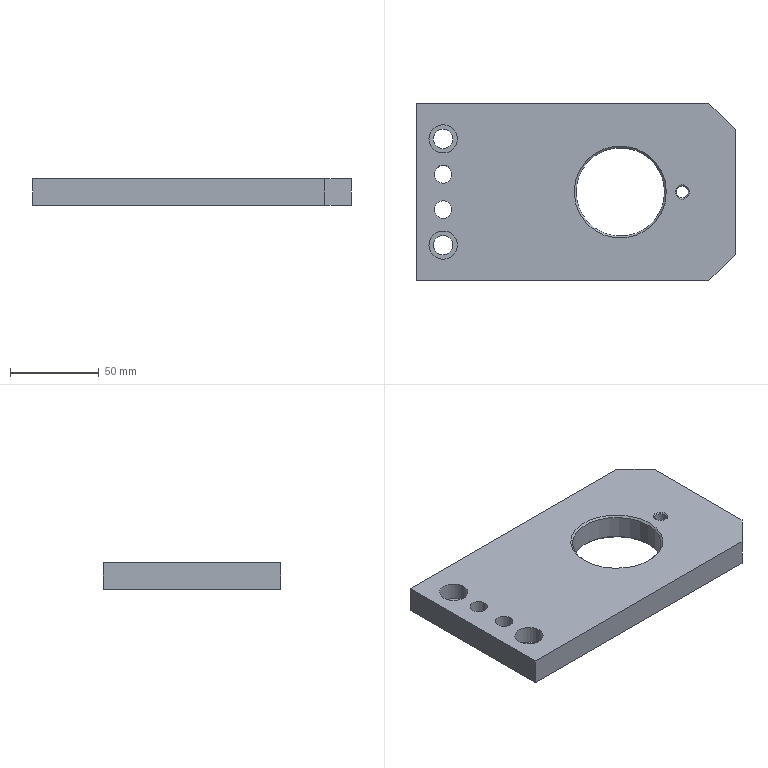Part | NX | features DATUM_CSYS 8, SKETCH 7, HOLE PACKAGE 5, EXTRACT_FACE 4, SIMPLE HOLE 3, CBORE_HOLE 2, CHAMFER 2, EXTRUDE 2, Instance Feature 1, Mirror Feature 1, SYMBOLIC_THREAD 1 | 1 solid | 22 faces | box 180 x 100 x 15 mm | volume 229133 mm3 | plane 10 | cylinder 8 | cone 4 | commonest cylinder face diameters 10 x2 11 x2 16 x2 6.8 x1 50 x1
STEP:
#1=CARTESIAN_POINT('',(0.,100.,0.));
#2=VERTEX_POINT('',#1);
#3=CARTESIAN_POINT('',(0.,0.,0.));
#4=VERTEX_POINT('',#3);
#5=CARTESIAN_POINT('',(0.,100.,0.));
#6=DIRECTION('',(0.,-1.,0.));
#7=VECTOR('',#6,1000.);
#8=LINE('',#5,#7);
#9=EDGE_CURVE('',#2,#4,#8,.T.);
#10=ORIENTED_EDGE('',*,*,#9,.T.);
#11=CARTESIAN_POINT('',(0.,0.,15.));
#12=VERTEX_POINT('',#11);
#13=CARTESIAN_POINT('',(0.,0.,15.));
#14=DIRECTION('',(0.,0.,-1.));
#15=VECTOR('',#14,1000.);
#16=LINE('',#13,#15);
#17=EDGE_CURVE('',#12,#4,#16,.T.);
#18=ORIENTED_EDGE('',*,*,#17,.F.);
#19=CARTESIAN_POINT('',(0.,100.,15.));
#20=VERTEX_POINT('',#19);
#21=CARTESIAN_POINT('',(0.,100.,15.));
#22=DIRECTION('',(0.,-1.,0.));
#23=VECTOR('',#22,1000.);
#24=LINE('',#21,#23);
#25=EDGE_CURVE('',#20,#12,#24,.T.);
#26=ORIENTED_EDGE('',*,*,#25,.F.);
#27=CARTESIAN_POINT('',(0.,100.,15.));
#28=DIRECTION('',(0.,0.,-1.));
#29=VECTOR('',#28,1000.);
#30=LINE('',#27,#29);
#31=EDGE_CURVE('',#20,#2,#30,.T.);
#32=ORIENTED_EDGE('',*,*,#31,.T.);
#33=EDGE_LOOP('',(#10,#18,#26,#32));
#34=FACE_BOUND('',#33,.T.);
#35=CARTESIAN_POINT('',(0.,100.,15.));
#36=DIRECTION('',(1.,0.,0.));
#37=DIRECTION('',(0.,0.,-1.));
#38=AXIS2_PLACEMENT_3D('',#35,#36,#37);
#39=PLANE('',#38);
#40=ADVANCED_FACE('',(#34),#39,.F.);
#41=CARTESIAN_POINT('',(165.,0.,0.));
#42=VERTEX_POINT('',#41);
#43=CARTESIAN_POINT('',(0.,0.,0.));
#44=DIRECTION('',(1.,0.,0.));
#45=VECTOR('',#44,1000.);
#46=LINE('',#43,#45);
#47=EDGE_CURVE('',#4,#42,#46,.T.);
#48=ORIENTED_EDGE('',*,*,#47,.T.);
#49=CARTESIAN_POINT('',(165.,0.,15.));
#50=VERTEX_POINT('',#49);
#51=CARTESIAN_POINT('',(165.,0.,15.));
#52=DIRECTION('',(0.,0.,1.));
#53=VECTOR('',#52,1000.);
#54=LINE('',#51,#53);
#55=EDGE_CURVE('',#42,#50,#54,.T.);
#56=ORIENTED_EDGE('',*,*,#55,.T.);
#57=CARTESIAN_POINT('',(0.,0.,15.));
#58=DIRECTION('',(1.,0.,0.));
#59=VECTOR('',#58,1000.);
#60=LINE('',#57,#59);
#61=EDGE_CURVE('',#12,#50,#60,.T.);
#62=ORIENTED_EDGE('',*,*,#61,.F.);
#63=ORIENTED_EDGE('',*,*,#17,.T.);
#64=EDGE_LOOP('',(#48,#56,#62,#63));
#65=FACE_BOUND('',#64,.T.);
#66=CARTESIAN_POINT('',(0.,0.,15.));
#67=DIRECTION('',(0.,1.,0.));
#68=DIRECTION('',(0.,0.,1.));
#69=AXIS2_PLACEMENT_3D('',#66,#67,#68);
#70=PLANE('',#69);
#71=ADVANCED_FACE('',(#65),#70,.F.);
#72=CARTESIAN_POINT('',(180.,15.,15.));
#73=VERTEX_POINT('',#72);
#74=CARTESIAN_POINT('',(180.,85.,15.));
#75=VERTEX_POINT('',#74);
#76=CARTESIAN_POINT('',(180.,0.,15.));
#77=DIRECTION('',(0.,1.,0.));
#78=VECTOR('',#77,1000.);
#79=LINE('',#76,#78);
#80=EDGE_CURVE('',#73,#75,#79,.T.);
#81=ORIENTED_EDGE('',*,*,#80,.F.);
#82=CARTESIAN_POINT('',(180.,15.,0.));
#83=VERTEX_POINT('',#82);
#84=CARTESIAN_POINT('',(180.,15.,15.));
#85=DIRECTION('',(0.,0.,-1.));
#86=VECTOR('',#85,1000.);
#87=LINE('',#84,#86);
#88=EDGE_CURVE('',#73,#83,#87,.T.);
#89=ORIENTED_EDGE('',*,*,#88,.T.);
#90=CARTESIAN_POINT('',(180.,85.,0.));
#91=VERTEX_POINT('',#90);
#92=CARTESIAN_POINT('',(180.,0.,0.));
#93=DIRECTION('',(0.,1.,0.));
#94=VECTOR('',#93,1000.);
#95=LINE('',#92,#94);
#96=EDGE_CURVE('',#83,#91,#95,.T.);
#97=ORIENTED_EDGE('',*,*,#96,.T.);
#98=CARTESIAN_POINT('',(180.,85.,15.));
#99=DIRECTION('',(0.,0.,1.));
#100=VECTOR('',#99,1000.);
#101=LINE('',#98,#100);
#102=EDGE_CURVE('',#91,#75,#101,.T.);
#103=ORIENTED_EDGE('',*,*,#102,.T.);
#104=EDGE_LOOP('',(#81,#89,#97,#103));
#105=FACE_BOUND('',#104,.T.);
#106=CARTESIAN_POINT('',(180.,0.,15.));
#107=DIRECTION('',(-1.,0.,0.));
#108=DIRECTION('',(0.,0.,1.));
#109=AXIS2_PLACEMENT_3D('',#106,#107,#108);
#110=PLANE('',#109);
#111=ADVANCED_FACE('',(#105),#110,.F.);
#112=CARTESIAN_POINT('',(165.,100.,15.));
#113=VERTEX_POINT('',#112);
#114=CARTESIAN_POINT('',(180.,100.,15.));
#115=DIRECTION('',(-1.,0.,0.));
#116=VECTOR('',#115,1000.);
#117=LINE('',#114,#116);
#118=EDGE_CURVE('',#113,#20,#117,.T.);
#119=ORIENTED_EDGE('',*,*,#118,.F.);
#120=CARTESIAN_POINT('',(165.,100.,0.));
#121=VERTEX_POINT('',#120);
#122=CARTESIAN_POINT('',(165.,100.,15.));
#123=DIRECTION('',(0.,0.,-1.));
#124=VECTOR('',#123,1000.);
#125=LINE('',#122,#124);
#126=EDGE_CURVE('',#113,#121,#125,.T.);
#127=ORIENTED_EDGE('',*,*,#126,.T.);
#128=CARTESIAN_POINT('',(180.,100.,0.));
#129=DIRECTION('',(-1.,0.,0.));
#130=VECTOR('',#129,1000.);
#131=LINE('',#128,#130);
#132=EDGE_CURVE('',#121,#2,#131,.T.);
#133=ORIENTED_EDGE('',*,*,#132,.T.);
#134=ORIENTED_EDGE('',*,*,#31,.F.);
#135=EDGE_LOOP('',(#119,#127,#133,#134));
#136=FACE_BOUND('',#135,.T.);
#137=CARTESIAN_POINT('',(180.,100.,15.));
#138=DIRECTION('',(0.,-1.,0.));
#139=DIRECTION('',(0.,0.,-1.));
#140=AXIS2_PLACEMENT_3D('',#137,#138,#139);
#141=PLANE('',#140);
#142=ADVANCED_FACE('',(#136),#141,.F.);
#143=CARTESIAN_POINT('',(10.,40.,15.));
#144=VERTEX_POINT('',#143);
#145=CARTESIAN_POINT('',(15.,40.,15.));
#146=DIRECTION('',(0.,0.,-1.));
#147=DIRECTION('',(-1.,0.,0.));
#148=AXIS2_PLACEMENT_3D('',#145,#146,#147);
#149=CIRCLE('',#148,5.);
#150=EDGE_CURVE('',#144,#144,#149,.T.);
#151=ORIENTED_EDGE('',*,*,#150,.T.);
#152=EDGE_LOOP('',(#151));
#153=FACE_BOUND('',#152,.T.);
#154=CARTESIAN_POINT('',(7.,20.,15.));
#155=VERTEX_POINT('',#154);
#156=CARTESIAN_POINT('',(15.,20.,15.));
#157=DIRECTION('',(0.,0.,-1.));
#158=DIRECTION('',(-1.,0.,0.));
#159=AXIS2_PLACEMENT_3D('',#156,#157,#158);
#160=CIRCLE('',#159,8.);
#161=EDGE_CURVE('',#155,#155,#160,.T.);
#162=ORIENTED_EDGE('',*,*,#161,.T.);
#163=EDGE_LOOP('',(#162));
#164=FACE_BOUND('',#163,.T.);
#165=CARTESIAN_POINT('',(10.,60.,15.));
#166=VERTEX_POINT('',#165);
#167=CARTESIAN_POINT('',(15.,60.,15.));
#168=DIRECTION('',(0.,0.,-1.));
#169=DIRECTION('',(-1.,0.,0.));
#170=AXIS2_PLACEMENT_3D('',#167,#168,#169);
#171=CIRCLE('',#170,5.);
#172=EDGE_CURVE('',#166,#166,#171,.T.);
#173=ORIENTED_EDGE('',*,*,#172,.T.);
#174=EDGE_LOOP('',(#173));
#175=FACE_BOUND('',#174,.T.);
#176=CARTESIAN_POINT('',(7.,80.,15.));
#177=VERTEX_POINT('',#176);
#178=CARTESIAN_POINT('',(15.,80.,15.));
#179=DIRECTION('',(0.,0.,-1.));
#180=DIRECTION('',(-1.,0.,0.));
#181=AXIS2_PLACEMENT_3D('',#178,#179,#180);
#182=CIRCLE('',#181,8.);
#183=EDGE_CURVE('',#177,#177,#182,.T.);
#184=ORIENTED_EDGE('',*,*,#183,.T.);
#185=EDGE_LOOP('',(#184));
#186=FACE_BOUND('',#185,.T.);
#187=CARTESIAN_POINT('',(154.,50.,15.));
#188=VERTEX_POINT('',#187);
#189=CARTESIAN_POINT('',(150.,50.,15.));
#190=DIRECTION('',(0.,0.,1.));
#191=DIRECTION('',(1.,0.,0.));
#192=AXIS2_PLACEMENT_3D('',#189,#190,#191);
#193=CIRCLE('',#192,4.);
#194=EDGE_CURVE('',#188,#188,#193,.F.);
#195=ORIENTED_EDGE('',*,*,#194,.T.);
#196=EDGE_LOOP('',(#195));
#197=FACE_BOUND('',#196,.T.);
#198=CARTESIAN_POINT('',(141.,50.,15.));
#199=VERTEX_POINT('',#198);
#200=CARTESIAN_POINT('',(115.,50.,15.));
#201=DIRECTION('',(0.,0.,1.));
#202=DIRECTION('',(1.,0.,0.));
#203=AXIS2_PLACEMENT_3D('',#200,#201,#202);
#204=CIRCLE('',#203,26.);
#205=EDGE_CURVE('',#199,#199,#204,.F.);
#206=ORIENTED_EDGE('',*,*,#205,.T.);
#207=EDGE_LOOP('',(#206));
#208=FACE_BOUND('',#207,.T.);
#209=ORIENTED_EDGE('',*,*,#61,.T.);
#210=CARTESIAN_POINT('',(82.5,-82.5,15.));
#211=DIRECTION('',(-0.7071,-0.7071,0.));
#212=VECTOR('',#211,1000.);
#213=LINE('',#210,#212);
#214=EDGE_CURVE('',#50,#73,#213,.F.);
#215=ORIENTED_EDGE('',*,*,#214,.T.);
#216=ORIENTED_EDGE('',*,*,#80,.T.);
#217=CARTESIAN_POINT('',(132.5,132.5,15.));
#218=DIRECTION('',(0.7071,-0.7071,0.));
#219=VECTOR('',#218,1000.);
#220=LINE('',#217,#219);
#221=EDGE_CURVE('',#75,#113,#220,.F.);
#222=ORIENTED_EDGE('',*,*,#221,.T.);
#223=ORIENTED_EDGE('',*,*,#118,.T.);
#224=ORIENTED_EDGE('',*,*,#25,.T.);
#225=EDGE_LOOP('',(#209,#215,#216,#222,#223,#224));
#226=FACE_BOUND('',#225,.T.);
#227=CARTESIAN_POINT('',(0.,0.,15.));
#228=DIRECTION('',(0.,0.,1.));
#229=DIRECTION('',(1.,0.,0.));
#230=AXIS2_PLACEMENT_3D('',#227,#228,#229);
#231=PLANE('',#230);
#232=ADVANCED_FACE('',(#153,#164,#175,#186,#197,#208,#226),#231,.T.);
#233=CARTESIAN_POINT('',(20.,40.,0.));
#234=VERTEX_POINT('',#233);
#235=CARTESIAN_POINT('',(15.,40.,0.));
#236=DIRECTION('',(0.,0.,1.));
#237=DIRECTION('',(1.,0.,0.));
#238=AXIS2_PLACEMENT_3D('',#235,#236,#237);
#239=CIRCLE('',#238,5.);
#240=EDGE_CURVE('',#234,#234,#239,.T.);
#241=ORIENTED_EDGE('',*,*,#240,.T.);
#242=EDGE_LOOP('',(#241));
#243=FACE_BOUND('',#242,.T.);
#244=CARTESIAN_POINT('',(20.5,20.,0.));
#245=VERTEX_POINT('',#244);
#246=CARTESIAN_POINT('',(15.,20.,0.));
#247=DIRECTION('',(0.,0.,1.));
#248=DIRECTION('',(1.,0.,0.));
#249=AXIS2_PLACEMENT_3D('',#246,#247,#248);
#250=CIRCLE('',#249,5.5);
#251=EDGE_CURVE('',#245,#245,#250,.T.);
#252=ORIENTED_EDGE('',*,*,#251,.T.);
#253=EDGE_LOOP('',(#252));
#254=FACE_BOUND('',#253,.T.);
#255=CARTESIAN_POINT('',(20.,60.,0.));
#256=VERTEX_POINT('',#255);
#257=CARTESIAN_POINT('',(15.,60.,0.));
#258=DIRECTION('',(0.,0.,1.));
#259=DIRECTION('',(1.,0.,0.));
#260=AXIS2_PLACEMENT_3D('',#257,#258,#259);
#261=CIRCLE('',#260,5.);
#262=EDGE_CURVE('',#256,#256,#261,.T.);
#263=ORIENTED_EDGE('',*,*,#262,.T.);
#264=EDGE_LOOP('',(#263));
#265=FACE_BOUND('',#264,.T.);
#266=CARTESIAN_POINT('',(20.5,80.,0.));
#267=VERTEX_POINT('',#266);
#268=CARTESIAN_POINT('',(15.,80.,0.));
#269=DIRECTION('',(0.,0.,1.));
#270=DIRECTION('',(1.,0.,0.));
#271=AXIS2_PLACEMENT_3D('',#268,#269,#270);
#272=CIRCLE('',#271,5.5);
#273=EDGE_CURVE('',#267,#267,#272,.T.);
#274=ORIENTED_EDGE('',*,*,#273,.T.);
#275=EDGE_LOOP('',(#274));
#276=FACE_BOUND('',#275,.T.);
#277=CARTESIAN_POINT('',(154.,50.,0.));
#278=VERTEX_POINT('',#277);
#279=CARTESIAN_POINT('',(150.,50.,0.));
#280=DIRECTION('',(0.,0.,1.));
#281=DIRECTION('',(1.,0.,0.));
#282=AXIS2_PLACEMENT_3D('',#279,#280,#281);
#283=CIRCLE('',#282,4.);
#284=EDGE_CURVE('',#278,#278,#283,.T.);
#285=ORIENTED_EDGE('',*,*,#284,.T.);
#286=EDGE_LOOP('',(#285));
#287=FACE_BOUND('',#286,.T.);
#288=CARTESIAN_POINT('',(141.,50.,0.));
#289=VERTEX_POINT('',#288);
#290=CARTESIAN_POINT('',(115.,50.,0.));
#291=DIRECTION('',(0.,0.,1.));
#292=DIRECTION('',(1.,0.,0.));
#293=AXIS2_PLACEMENT_3D('',#290,#291,#292);
#294=CIRCLE('',#293,26.);
#295=EDGE_CURVE('',#289,#289,#294,.T.);
#296=ORIENTED_EDGE('',*,*,#295,.T.);
#297=EDGE_LOOP('',(#296));
#298=FACE_BOUND('',#297,.T.);
#299=ORIENTED_EDGE('',*,*,#96,.F.);
#300=CARTESIAN_POINT('',(180.,15.,0.));
#301=DIRECTION('',(0.7071,0.7071,0.));
#302=VECTOR('',#301,1000.);
#303=LINE('',#300,#302);
#304=EDGE_CURVE('',#83,#42,#303,.F.);
#305=ORIENTED_EDGE('',*,*,#304,.T.);
#306=ORIENTED_EDGE('',*,*,#47,.F.);
#307=ORIENTED_EDGE('',*,*,#9,.F.);
#308=ORIENTED_EDGE('',*,*,#132,.F.);
#309=CARTESIAN_POINT('',(165.,100.,0.));
#310=DIRECTION('',(-0.7071,0.7071,0.));
#311=VECTOR('',#310,1000.);
#312=LINE('',#309,#311);
#313=EDGE_CURVE('',#121,#91,#312,.F.);
#314=ORIENTED_EDGE('',*,*,#313,.T.);
#315=EDGE_LOOP('',(#299,#305,#306,#307,#308,#314));
#316=FACE_BOUND('',#315,.T.);
#317=CARTESIAN_POINT('',(0.,0.,0.));
#318=DIRECTION('',(0.,0.,1.));
#319=DIRECTION('',(1.,0.,0.));
#320=AXIS2_PLACEMENT_3D('',#317,#318,#319);
#321=PLANE('',#320);
#322=ADVANCED_FACE('',(#243,#254,#265,#276,#287,#298,#316),#321,.F.);
#323=CARTESIAN_POINT('',(140.,50.,1.));
#324=VERTEX_POINT('',#323);
#325=CARTESIAN_POINT('',(115.,50.,1.));
#326=DIRECTION('',(0.,0.,1.));
#327=DIRECTION('',(1.,0.,0.));
#328=AXIS2_PLACEMENT_3D('',#325,#326,#327);
#329=CIRCLE('',#328,25.);
#330=EDGE_CURVE('',#324,#324,#329,.F.);
#331=ORIENTED_EDGE('',*,*,#330,.T.);
#332=EDGE_LOOP('',(#331));
#333=FACE_BOUND('',#332,.T.);
#334=CARTESIAN_POINT('',(140.,50.,14.));
#335=VERTEX_POINT('',#334);
#336=CARTESIAN_POINT('',(115.,50.,14.));
#337=DIRECTION('',(0.,0.,1.));
#338=DIRECTION('',(1.,0.,0.));
#339=AXIS2_PLACEMENT_3D('',#336,#337,#338);
#340=CIRCLE('',#339,25.);
#341=EDGE_CURVE('',#335,#335,#340,.T.);
#342=ORIENTED_EDGE('',*,*,#341,.T.);
#343=EDGE_LOOP('',(#342));
#344=FACE_BOUND('',#343,.T.);
#345=CARTESIAN_POINT('',(115.,50.,-81.));
#346=DIRECTION('',(0.,0.,1.));
#347=DIRECTION('',(1.,0.,0.));
#348=AXIS2_PLACEMENT_3D('',#345,#346,#347);
#349=CYLINDRICAL_SURFACE('',#348,25.);
#350=ADVANCED_FACE('',(#333,#344),#349,.F.);
#351=ORIENTED_EDGE('',*,*,#214,.F.);
#352=ORIENTED_EDGE('',*,*,#55,.F.);
#353=ORIENTED_EDGE('',*,*,#304,.F.);
#354=ORIENTED_EDGE('',*,*,#88,.F.);
#355=EDGE_LOOP('',(#351,#352,#353,#354));
#356=FACE_BOUND('',#355,.T.);
#357=CARTESIAN_POINT('',(180.,15.,15.));
#358=DIRECTION('',(-0.7071,0.7071,0.));
#359=DIRECTION('',(0.,0.,-1.));
#360=AXIS2_PLACEMENT_3D('',#357,#358,#359);
#361=PLANE('',#360);
#362=ADVANCED_FACE('',(#356),#361,.F.);
#363=ORIENTED_EDGE('',*,*,#221,.F.);
#364=ORIENTED_EDGE('',*,*,#102,.F.);
#365=ORIENTED_EDGE('',*,*,#313,.F.);
#366=ORIENTED_EDGE('',*,*,#126,.F.);
#367=EDGE_LOOP('',(#363,#364,#365,#366));
#368=FACE_BOUND('',#367,.T.);
#369=CARTESIAN_POINT('',(165.,100.,15.));
#370=DIRECTION('',(-0.7071,-0.7071,0.));
#371=DIRECTION('',(0.,0.,-1.));
#372=AXIS2_PLACEMENT_3D('',#369,#370,#371);
#373=PLANE('',#372);
#374=ADVANCED_FACE('',(#368),#373,.F.);
#375=ORIENTED_EDGE('',*,*,#330,.F.);
#376=EDGE_LOOP('',(#375));
#377=FACE_BOUND('',#376,.T.);
#378=ORIENTED_EDGE('',*,*,#295,.F.);
#379=EDGE_LOOP('',(#378));
#380=FACE_BOUND('',#379,.T.);
#381=CARTESIAN_POINT('',(115.,50.,0.));
#382=DIRECTION('',(0.,0.,-1.));
#383=DIRECTION('',(-1.,0.,0.));
#384=AXIS2_PLACEMENT_3D('',#381,#382,#383);
#385=CONICAL_SURFACE('',#384,26.,0.7854);
#386=ADVANCED_FACE('',(#377,#380),#385,.F.);
#387=ORIENTED_EDGE('',*,*,#205,.F.);
#388=EDGE_LOOP('',(#387));
#389=FACE_BOUND('',#388,.T.);
#390=ORIENTED_EDGE('',*,*,#341,.F.);
#391=EDGE_LOOP('',(#390));
#392=FACE_BOUND('',#391,.T.);
#393=CARTESIAN_POINT('',(115.,50.,14.));
#394=DIRECTION('',(0.,0.,1.));
#395=DIRECTION('',(1.,0.,0.));
#396=AXIS2_PLACEMENT_3D('',#393,#394,#395);
#397=CONICAL_SURFACE('',#396,25.,0.7854);
#398=ADVANCED_FACE('',(#389,#392),#397,.F.);
#399=CARTESIAN_POINT('',(153.4,50.,0.6));
#400=VERTEX_POINT('',#399);
#401=CARTESIAN_POINT('',(150.,50.,0.6));
#402=DIRECTION('',(0.,0.,1.));
#403=DIRECTION('',(1.,0.,0.));
#404=AXIS2_PLACEMENT_3D('',#401,#402,#403);
#405=CIRCLE('',#404,3.4);
#406=EDGE_CURVE('',#400,#400,#405,.F.);
#407=ORIENTED_EDGE('',*,*,#406,.T.);
#408=EDGE_LOOP('',(#407));
#409=FACE_BOUND('',#408,.T.);
#410=CARTESIAN_POINT('',(153.4,50.,14.4));
#411=VERTEX_POINT('',#410);
#412=CARTESIAN_POINT('',(150.,50.,14.4));
#413=DIRECTION('',(0.,0.,1.));
#414=DIRECTION('',(1.,0.,0.));
#415=AXIS2_PLACEMENT_3D('',#412,#413,#414);
#416=CIRCLE('',#415,3.4);
#417=EDGE_CURVE('',#411,#411,#416,.T.);
#418=ORIENTED_EDGE('',*,*,#417,.T.);
#419=EDGE_LOOP('',(#418));
#420=FACE_BOUND('',#419,.T.);
#421=CARTESIAN_POINT('',(150.,50.,15.));
#422=DIRECTION('',(0.,0.,-1.));
#423=DIRECTION('',(-1.,0.,0.));
#424=AXIS2_PLACEMENT_3D('',#421,#422,#423);
#425=CYLINDRICAL_SURFACE('',#424,3.4);
#426=ADVANCED_FACE('',(#409,#420),#425,.F.);
#427=ORIENTED_EDGE('',*,*,#417,.F.);
#428=EDGE_LOOP('',(#427));
#429=FACE_BOUND('',#428,.T.);
#430=ORIENTED_EDGE('',*,*,#194,.F.);
#431=EDGE_LOOP('',(#430));
#432=FACE_BOUND('',#431,.T.);
#433=CARTESIAN_POINT('',(150.,50.,15.));
#434=DIRECTION('',(0.,0.,1.));
#435=DIRECTION('',(1.,0.,0.));
#436=AXIS2_PLACEMENT_3D('',#433,#434,#435);
#437=CONICAL_SURFACE('',#436,4.,0.7854);
#438=ADVANCED_FACE('',(#429,#432),#437,.F.);
#439=ORIENTED_EDGE('',*,*,#406,.F.);
#440=EDGE_LOOP('',(#439));
#441=FACE_BOUND('',#440,.T.);
#442=ORIENTED_EDGE('',*,*,#284,.F.);
#443=EDGE_LOOP('',(#442));
#444=FACE_BOUND('',#443,.T.);
#445=CARTESIAN_POINT('',(150.,50.,0.));
#446=DIRECTION('',(0.,0.,-1.));
#447=DIRECTION('',(-1.,0.,0.));
#448=AXIS2_PLACEMENT_3D('',#445,#446,#447);
#449=CONICAL_SURFACE('',#448,4.,0.7854);
#450=ADVANCED_FACE('',(#441,#444),#449,.F.);
#451=CARTESIAN_POINT('',(9.5,80.,5.));
#452=VERTEX_POINT('',#451);
#453=CARTESIAN_POINT('',(15.,80.,5.));
#454=DIRECTION('',(0.,0.,-1.));
#455=DIRECTION('',(-1.,0.,0.));
#456=AXIS2_PLACEMENT_3D('',#453,#454,#455);
#457=CIRCLE('',#456,5.5);
#458=EDGE_CURVE('',#452,#452,#457,.F.);
#459=ORIENTED_EDGE('',*,*,#458,.T.);
#460=EDGE_LOOP('',(#459));
#461=FACE_BOUND('',#460,.T.);
#462=ORIENTED_EDGE('',*,*,#273,.F.);
#463=EDGE_LOOP('',(#462));
#464=FACE_BOUND('',#463,.T.);
#465=CARTESIAN_POINT('',(15.,80.,-485.));
#466=DIRECTION('',(0.,0.,-1.));
#467=DIRECTION('',(-1.,0.,0.));
#468=AXIS2_PLACEMENT_3D('',#465,#466,#467);
#469=CYLINDRICAL_SURFACE('',#468,5.5);
#470=ADVANCED_FACE('',(#461,#464),#469,.F.);
#471=ORIENTED_EDGE('',*,*,#458,.F.);
#472=EDGE_LOOP('',(#471));
#473=FACE_BOUND('',#472,.T.);
#474=CARTESIAN_POINT('',(7.,80.,5.));
#475=VERTEX_POINT('',#474);
#476=CARTESIAN_POINT('',(15.,80.,5.));
#477=DIRECTION('',(0.,0.,-1.));
#478=DIRECTION('',(-1.,0.,0.));
#479=AXIS2_PLACEMENT_3D('',#476,#477,#478);
#480=CIRCLE('',#479,8.);
#481=EDGE_CURVE('',#475,#475,#480,.F.);
#482=ORIENTED_EDGE('',*,*,#481,.T.);
#483=EDGE_LOOP('',(#482));
#484=FACE_BOUND('',#483,.T.);
#485=CARTESIAN_POINT('',(15.,80.,5.));
#486=DIRECTION('',(0.,0.,-1.));
#487=DIRECTION('',(-1.,0.,0.));
#488=AXIS2_PLACEMENT_3D('',#485,#486,#487);
#489=PLANE('',#488);
#490=ADVANCED_FACE('',(#473,#484),#489,.F.);
#491=ORIENTED_EDGE('',*,*,#481,.F.);
#492=EDGE_LOOP('',(#491));
#493=FACE_BOUND('',#492,.T.);
#494=ORIENTED_EDGE('',*,*,#183,.F.);
#495=EDGE_LOOP('',(#494));
#496=FACE_BOUND('',#495,.T.);
#497=CARTESIAN_POINT('',(15.,80.,15.));
#498=DIRECTION('',(0.,0.,-1.));
#499=DIRECTION('',(-1.,0.,0.));
#500=AXIS2_PLACEMENT_3D('',#497,#498,#499);
#501=CYLINDRICAL_SURFACE('',#500,8.);
#502=ADVANCED_FACE('',(#493,#496),#501,.F.);
#503=ORIENTED_EDGE('',*,*,#172,.F.);
#504=EDGE_LOOP('',(#503));
#505=FACE_BOUND('',#504,.T.);
#506=ORIENTED_EDGE('',*,*,#262,.F.);
#507=EDGE_LOOP('',(#506));
#508=FACE_BOUND('',#507,.T.);
#509=CARTESIAN_POINT('',(15.,60.,15.));
#510=DIRECTION('',(0.,0.,-1.));
#511=DIRECTION('',(-1.,0.,0.));
#512=AXIS2_PLACEMENT_3D('',#509,#510,#511);
#513=CYLINDRICAL_SURFACE('',#512,5.);
#514=ADVANCED_FACE('',(#505,#508),#513,.F.);
#515=CARTESIAN_POINT('',(9.5,20.,5.));
#516=VERTEX_POINT('',#515);
#517=CARTESIAN_POINT('',(15.,20.,5.));
#518=DIRECTION('',(0.,0.,-1.));
#519=DIRECTION('',(-1.,0.,0.));
#520=AXIS2_PLACEMENT_3D('',#517,#518,#519);
#521=CIRCLE('',#520,5.5);
#522=EDGE_CURVE('',#516,#516,#521,.T.);
#523=ORIENTED_EDGE('',*,*,#522,.F.);
#524=EDGE_LOOP('',(#523));
#525=FACE_BOUND('',#524,.T.);
#526=ORIENTED_EDGE('',*,*,#251,.F.);
#527=EDGE_LOOP('',(#526));
#528=FACE_BOUND('',#527,.T.);
#529=CARTESIAN_POINT('',(15.,20.,-485.));
#530=DIRECTION('',(0.,0.,-1.));
#531=DIRECTION('',(-1.,0.,0.));
#532=AXIS2_PLACEMENT_3D('',#529,#530,#531);
#533=CYLINDRICAL_SURFACE('',#532,5.5);
#534=ADVANCED_FACE('',(#525,#528),#533,.F.);
#535=ORIENTED_EDGE('',*,*,#522,.T.);
#536=EDGE_LOOP('',(#535));
#537=FACE_BOUND('',#536,.T.);
#538=CARTESIAN_POINT('',(7.,20.,5.));
#539=VERTEX_POINT('',#538);
#540=CARTESIAN_POINT('',(15.,20.,5.));
#541=DIRECTION('',(0.,0.,-1.));
#542=DIRECTION('',(-1.,0.,0.));
#543=AXIS2_PLACEMENT_3D('',#540,#541,#542);
#544=CIRCLE('',#543,8.);
#545=EDGE_CURVE('',#539,#539,#544,.T.);
#546=ORIENTED_EDGE('',*,*,#545,.F.);
#547=EDGE_LOOP('',(#546));
#548=FACE_BOUND('',#547,.T.);
#549=CARTESIAN_POINT('',(15.,20.,5.));
#550=DIRECTION('',(0.,0.,-1.));
#551=DIRECTION('',(-1.,0.,0.));
#552=AXIS2_PLACEMENT_3D('',#549,#550,#551);
#553=PLANE('',#552);
#554=ADVANCED_FACE('',(#537,#548),#553,.F.);
#555=ORIENTED_EDGE('',*,*,#545,.T.);
#556=EDGE_LOOP('',(#555));
#557=FACE_BOUND('',#556,.T.);
#558=ORIENTED_EDGE('',*,*,#161,.F.);
#559=EDGE_LOOP('',(#558));
#560=FACE_BOUND('',#559,.T.);
#561=CARTESIAN_POINT('',(15.,20.,15.));
#562=DIRECTION('',(0.,0.,-1.));
#563=DIRECTION('',(-1.,0.,0.));
#564=AXIS2_PLACEMENT_3D('',#561,#562,#563);
#565=CYLINDRICAL_SURFACE('',#564,8.);
#566=ADVANCED_FACE('',(#557,#560),#565,.F.);
#567=ORIENTED_EDGE('',*,*,#150,.F.);
#568=EDGE_LOOP('',(#567));
#569=FACE_BOUND('',#568,.T.);
#570=ORIENTED_EDGE('',*,*,#240,.F.);
#571=EDGE_LOOP('',(#570));
#572=FACE_BOUND('',#571,.T.);
#573=CARTESIAN_POINT('',(15.,40.,15.));
#574=DIRECTION('',(0.,0.,-1.));
#575=DIRECTION('',(-1.,0.,0.));
#576=AXIS2_PLACEMENT_3D('',#573,#574,#575);
#577=CYLINDRICAL_SURFACE('',#576,5.);
#578=ADVANCED_FACE('',(#569,#572),#577,.F.);
#579=CLOSED_SHELL('',(#40,#71,#111,#142,#232,#322,#350,#362,#374,#386,#398,#426,#438,#450,#470,#490,#502,#514,#534,#554,#566,#578));
#580=MANIFOLD_SOLID_BREP('',#579);
#581=(LENGTH_UNIT()NAMED_UNIT(*)SI_UNIT(.MILLI.,.METRE.));
#582=UNCERTAINTY_MEASURE_WITH_UNIT(LENGTH_MEASURE(0.00001),#581,'','');
#583=(NAMED_UNIT(*)PLANE_ANGLE_UNIT()SI_UNIT($,.RADIAN.));
#584=(NAMED_UNIT(*)SI_UNIT($,.STERADIAN.)SOLID_ANGLE_UNIT());
#585=(GEOMETRIC_REPRESENTATION_CONTEXT(3)GLOBAL_UNCERTAINTY_ASSIGNED_CONTEXT((#582))GLOBAL_UNIT_ASSIGNED_CONTEXT((#581,#583,#584))REPRESENTATION_CONTEXT('',''));
#586=ADVANCED_BREP_SHAPE_REPRESENTATION('',(#580),#585);